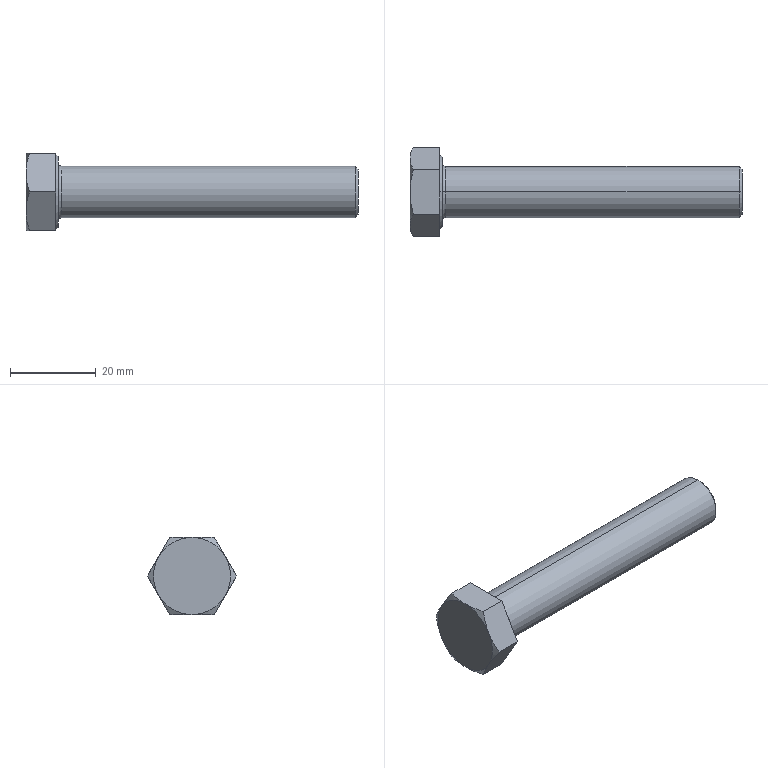Part | SolidWorks | features Chamfer 2, RevCut 2, Revolution 2, Extrusion 1, ICE 1 | 1 solid | 24 faces | box 77.5 x 20.785 x 18 mm | volume 9981 mm3 | cone 10 | plane 10 | cylinder 2 | torus 2 | commonest cylinder face diameters 12 x2
STEP:
#1=CARTESIAN_POINT('',(7.5,0.,8.215));
#2=VERTEX_POINT('',#1);
#3=CARTESIAN_POINT('',(7.5,0.,-8.215));
#4=VERTEX_POINT('',#3);
#5=CARTESIAN_POINT('',(7.5,0.,0.));
#6=DIRECTION('',(-1.,0.,0.));
#7=DIRECTION('',(0.,0.,1.));
#8=AXIS2_PLACEMENT_3D('',#5,#6,#7);
#9=CIRCLE('',#8,8.215);
#10=EDGE_CURVE('',#2,#4,#9,.T.);
#11=ORIENTED_EDGE('',*,*,#10,.T.);
#12=CARTESIAN_POINT('',(6.9,0.,-8.815));
#13=VERTEX_POINT('',#12);
#14=CARTESIAN_POINT('',(6.9,0.,-8.815));
#15=DIRECTION('',(-0.7071,0.,-0.7071));
#16=VECTOR('',#15,1000.);
#17=LINE('',#14,#16);
#18=EDGE_CURVE('',#4,#13,#17,.T.);
#19=ORIENTED_EDGE('',*,*,#18,.T.);
#20=CARTESIAN_POINT('',(6.9,0.,8.815));
#21=VERTEX_POINT('',#20);
#22=CARTESIAN_POINT('',(6.9,0.,0.));
#23=DIRECTION('',(-1.,0.,0.));
#24=DIRECTION('',(0.,0.,1.));
#25=AXIS2_PLACEMENT_3D('',#22,#23,#24);
#26=CIRCLE('',#25,8.815);
#27=EDGE_CURVE('',#21,#13,#26,.T.);
#28=ORIENTED_EDGE('',*,*,#27,.F.);
#29=CARTESIAN_POINT('',(6.9,0.,8.815));
#30=DIRECTION('',(-0.7071,0.,0.7071));
#31=VECTOR('',#30,1000.);
#32=LINE('',#29,#31);
#33=EDGE_CURVE('',#2,#21,#32,.T.);
#34=ORIENTED_EDGE('',*,*,#33,.F.);
#35=EDGE_LOOP('',(#11,#19,#28,#34));
#36=FACE_OUTER_BOUND('',#35,.T.);
#37=CARTESIAN_POINT('',(6.9,0.,0.));
#38=DIRECTION('',(-1.,0.,0.));
#39=DIRECTION('',(0.,0.,1.));
#40=AXIS2_PLACEMENT_3D('',#37,#38,#39);
#41=CONICAL_SURFACE('',#40,8.815,0.7854);
#42=ADVANCED_FACE('',(#36),#41,.T.);
#43=CARTESIAN_POINT('',(77.5,0.,-5.333));
#44=VERTEX_POINT('',#43);
#45=CARTESIAN_POINT('',(77.5,0.,5.333));
#46=VERTEX_POINT('',#45);
#47=CARTESIAN_POINT('',(77.5,0.,0.));
#48=DIRECTION('',(1.,0.,0.));
#49=DIRECTION('',(0.,0.,1.));
#50=AXIS2_PLACEMENT_3D('',#47,#48,#49);
#51=CIRCLE('',#50,5.333);
#52=EDGE_CURVE('',#44,#46,#51,.T.);
#53=ORIENTED_EDGE('',*,*,#52,.F.);
#54=CARTESIAN_POINT('',(76.833,0.,-6.));
#55=VERTEX_POINT('',#54);
#56=CARTESIAN_POINT('',(76.833,0.,-6.));
#57=DIRECTION('',(-0.7071,0.,-0.7071));
#58=VECTOR('',#57,1000.);
#59=LINE('',#56,#58);
#60=EDGE_CURVE('',#44,#55,#59,.T.);
#61=ORIENTED_EDGE('',*,*,#60,.T.);
#62=CARTESIAN_POINT('',(76.833,0.,6.));
#63=VERTEX_POINT('',#62);
#64=CARTESIAN_POINT('',(76.833,0.,0.));
#65=DIRECTION('',(-1.,0.,0.));
#66=DIRECTION('',(0.,0.,1.));
#67=AXIS2_PLACEMENT_3D('',#64,#65,#66);
#68=CIRCLE('',#67,6.);
#69=EDGE_CURVE('',#63,#55,#68,.T.);
#70=ORIENTED_EDGE('',*,*,#69,.F.);
#71=CARTESIAN_POINT('',(76.833,0.,6.));
#72=DIRECTION('',(-0.7071,0.,0.7071));
#73=VECTOR('',#72,1000.);
#74=LINE('',#71,#73);
#75=EDGE_CURVE('',#46,#63,#74,.T.);
#76=ORIENTED_EDGE('',*,*,#75,.F.);
#77=EDGE_LOOP('',(#53,#61,#70,#76));
#78=FACE_OUTER_BOUND('',#77,.T.);
#79=CARTESIAN_POINT('',(76.833,0.,0.));
#80=DIRECTION('',(-1.,0.,0.));
#81=DIRECTION('',(0.,0.,1.));
#82=AXIS2_PLACEMENT_3D('',#79,#80,#81);
#83=CONICAL_SURFACE('',#82,6.,0.7854);
#84=ADVANCED_FACE('',(#78),#83,.T.);
#85=ORIENTED_EDGE('',*,*,#69,.T.);
#86=CARTESIAN_POINT('',(8.35,0.,-6.));
#87=VERTEX_POINT('',#86);
#88=CARTESIAN_POINT('',(7.5,0.,-6.));
#89=DIRECTION('',(-1.,0.,0.));
#90=VECTOR('',#89,1000.);
#91=LINE('',#88,#90);
#92=EDGE_CURVE('',#55,#87,#91,.T.);
#93=ORIENTED_EDGE('',*,*,#92,.T.);
#94=CARTESIAN_POINT('',(8.35,0.,6.));
#95=VERTEX_POINT('',#94);
#96=CARTESIAN_POINT('',(8.35,0.,0.));
#97=DIRECTION('',(-1.,0.,0.));
#98=DIRECTION('',(0.,0.,1.));
#99=AXIS2_PLACEMENT_3D('',#96,#97,#98);
#100=CIRCLE('',#99,6.);
#101=EDGE_CURVE('',#95,#87,#100,.T.);
#102=ORIENTED_EDGE('',*,*,#101,.F.);
#103=CARTESIAN_POINT('',(7.5,0.,6.));
#104=DIRECTION('',(-1.,0.,0.));
#105=VECTOR('',#104,1000.);
#106=LINE('',#103,#105);
#107=EDGE_CURVE('',#63,#95,#106,.T.);
#108=ORIENTED_EDGE('',*,*,#107,.F.);
#109=EDGE_LOOP('',(#85,#93,#102,#108));
#110=FACE_OUTER_BOUND('',#109,.T.);
#111=CARTESIAN_POINT('',(7.5,0.,0.));
#112=DIRECTION('',(-1.,0.,0.));
#113=DIRECTION('',(0.,0.,1.));
#114=AXIS2_PLACEMENT_3D('',#111,#112,#113);
#115=CYLINDRICAL_SURFACE('',#114,6.);
#116=ADVANCED_FACE('',(#110),#115,.T.);
#117=CARTESIAN_POINT('',(7.5,0.,-6.85));
#118=VERTEX_POINT('',#117);
#119=CARTESIAN_POINT('',(7.5,0.,6.85));
#120=VERTEX_POINT('',#119);
#121=CARTESIAN_POINT('',(7.5,0.,0.));
#122=DIRECTION('',(-1.,0.,0.));
#123=DIRECTION('',(0.,0.,1.));
#124=AXIS2_PLACEMENT_3D('',#121,#122,#123);
#125=CIRCLE('',#124,6.85);
#126=EDGE_CURVE('',#118,#120,#125,.T.);
#127=ORIENTED_EDGE('',*,*,#126,.F.);
#128=CARTESIAN_POINT('',(8.35,0.,-6.85));
#129=DIRECTION('',(0.,1.,0.));
#130=DIRECTION('',(0.,0.,1.));
#131=AXIS2_PLACEMENT_3D('',#128,#129,#130);
#132=CIRCLE('',#131,0.85);
#133=EDGE_CURVE('',#118,#87,#132,.T.);
#134=ORIENTED_EDGE('',*,*,#133,.T.);
#135=CARTESIAN_POINT('',(8.35,0.,0.));
#136=DIRECTION('',(-1.,0.,0.));
#137=DIRECTION('',(0.,0.,1.));
#138=AXIS2_PLACEMENT_3D('',#135,#136,#137);
#139=CIRCLE('',#138,6.);
#140=EDGE_CURVE('',#87,#95,#139,.T.);
#141=ORIENTED_EDGE('',*,*,#140,.T.);
#142=CARTESIAN_POINT('',(8.35,0.,6.85));
#143=DIRECTION('',(0.,-1.,0.));
#144=DIRECTION('',(0.,0.,-1.));
#145=AXIS2_PLACEMENT_3D('',#142,#143,#144);
#146=CIRCLE('',#145,0.85);
#147=EDGE_CURVE('',#120,#95,#146,.T.);
#148=ORIENTED_EDGE('',*,*,#147,.F.);
#149=EDGE_LOOP('',(#127,#134,#141,#148));
#150=FACE_OUTER_BOUND('',#149,.T.);
#151=CARTESIAN_POINT('',(8.35,0.,0.));
#152=DIRECTION('',(-1.,0.,0.));
#153=DIRECTION('',(0.,0.,1.));
#154=AXIS2_PLACEMENT_3D('',#151,#152,#153);
#155=TOROIDAL_SURFACE('',#154,6.85,0.85);
#156=ADVANCED_FACE('',(#150),#155,.F.);
#157=CARTESIAN_POINT('',(7.5,0.,0.));
#158=DIRECTION('',(-1.,0.,0.));
#159=DIRECTION('',(0.,0.,1.));
#160=AXIS2_PLACEMENT_3D('',#157,#158,#159);
#161=CIRCLE('',#160,6.85);
#162=EDGE_CURVE('',#120,#118,#161,.T.);
#163=ORIENTED_EDGE('',*,*,#162,.T.);
#164=ORIENTED_EDGE('',*,*,#126,.T.);
#165=EDGE_LOOP('',(#163,#164));
#166=FACE_BOUND('',#165,.T.);
#167=ORIENTED_EDGE('',*,*,#10,.F.);
#168=CARTESIAN_POINT('',(7.5,0.,0.));
#169=DIRECTION('',(-1.,0.,0.));
#170=DIRECTION('',(0.,0.,1.));
#171=AXIS2_PLACEMENT_3D('',#168,#169,#170);
#172=CIRCLE('',#171,8.215);
#173=EDGE_CURVE('',#4,#2,#172,.T.);
#174=ORIENTED_EDGE('',*,*,#173,.F.);
#175=EDGE_LOOP('',(#167,#174));
#176=FACE_OUTER_BOUND('',#175,.T.);
#177=CARTESIAN_POINT('',(7.5,5.196,-9.));
#178=DIRECTION('',(1.,0.,0.));
#179=DIRECTION('',(0.,0.,-1.));
#180=AXIS2_PLACEMENT_3D('',#177,#178,#179);
#181=PLANE('',#180);
#182=ADVANCED_FACE('',(#166,#176),#181,.T.);
#183=ORIENTED_EDGE('',*,*,#133,.F.);
#184=ORIENTED_EDGE('',*,*,#162,.F.);
#185=ORIENTED_EDGE('',*,*,#147,.T.);
#186=ORIENTED_EDGE('',*,*,#101,.T.);
#187=EDGE_LOOP('',(#183,#184,#185,#186));
#188=FACE_OUTER_BOUND('',#187,.T.);
#189=CARTESIAN_POINT('',(8.35,0.,0.));
#190=DIRECTION('',(-1.,0.,0.));
#191=DIRECTION('',(0.,0.,1.));
#192=AXIS2_PLACEMENT_3D('',#189,#190,#191);
#193=TOROIDAL_SURFACE('',#192,6.85,0.85);
#194=ADVANCED_FACE('',(#188),#193,.F.);
#195=CARTESIAN_POINT('',(77.5,0.,0.));
#196=DIRECTION('',(1.,0.,0.));
#197=DIRECTION('',(0.,0.,1.));
#198=AXIS2_PLACEMENT_3D('',#195,#196,#197);
#199=CIRCLE('',#198,5.333);
#200=EDGE_CURVE('',#46,#44,#199,.T.);
#201=ORIENTED_EDGE('',*,*,#200,.T.);
#202=ORIENTED_EDGE('',*,*,#52,.T.);
#203=EDGE_LOOP('',(#201,#202));
#204=FACE_OUTER_BOUND('',#203,.T.);
#205=CARTESIAN_POINT('',(77.5,6.,0.));
#206=DIRECTION('',(-1.,0.,0.));
#207=DIRECTION('',(0.,0.,1.));
#208=AXIS2_PLACEMENT_3D('',#205,#206,#207);
#209=PLANE('',#208);
#210=ADVANCED_FACE('',(#204),#209,.F.);
#211=ORIENTED_EDGE('',*,*,#92,.F.);
#212=CARTESIAN_POINT('',(76.833,0.,0.));
#213=DIRECTION('',(-1.,0.,0.));
#214=DIRECTION('',(0.,0.,1.));
#215=AXIS2_PLACEMENT_3D('',#212,#213,#214);
#216=CIRCLE('',#215,6.);
#217=EDGE_CURVE('',#55,#63,#216,.T.);
#218=ORIENTED_EDGE('',*,*,#217,.T.);
#219=ORIENTED_EDGE('',*,*,#107,.T.);
#220=ORIENTED_EDGE('',*,*,#140,.F.);
#221=EDGE_LOOP('',(#211,#218,#219,#220));
#222=FACE_OUTER_BOUND('',#221,.T.);
#223=CARTESIAN_POINT('',(7.5,0.,0.));
#224=DIRECTION('',(-1.,0.,0.));
#225=DIRECTION('',(0.,0.,1.));
#226=AXIS2_PLACEMENT_3D('',#223,#224,#225);
#227=CYLINDRICAL_SURFACE('',#226,6.);
#228=ADVANCED_FACE('',(#222),#227,.T.);
#229=ORIENTED_EDGE('',*,*,#60,.F.);
#230=ORIENTED_EDGE('',*,*,#200,.F.);
#231=ORIENTED_EDGE('',*,*,#75,.T.);
#232=ORIENTED_EDGE('',*,*,#217,.F.);
#233=EDGE_LOOP('',(#229,#230,#231,#232));
#234=FACE_OUTER_BOUND('',#233,.T.);
#235=CARTESIAN_POINT('',(76.833,0.,0.));
#236=DIRECTION('',(-1.,0.,0.));
#237=DIRECTION('',(0.,0.,1.));
#238=AXIS2_PLACEMENT_3D('',#235,#236,#237);
#239=CONICAL_SURFACE('',#238,6.,0.7854);
#240=ADVANCED_FACE('',(#234),#239,.T.);
#241=ORIENTED_EDGE('',*,*,#27,.T.);
#242=CARTESIAN_POINT('',(6.9,0.,0.));
#243=DIRECTION('',(-1.,0.,0.));
#244=DIRECTION('',(0.,0.,1.));
#245=AXIS2_PLACEMENT_3D('',#242,#243,#244);
#246=CIRCLE('',#245,8.815);
#247=EDGE_CURVE('',#13,#21,#246,.T.);
#248=ORIENTED_EDGE('',*,*,#247,.T.);
#249=EDGE_LOOP('',(#241,#248));
#250=FACE_BOUND('',#249,.T.);
#251=CARTESIAN_POINT('',(6.9,-5.196,-9.));
#252=VERTEX_POINT('',#251);
#253=CARTESIAN_POINT('',(6.9,5.196,-9.));
#254=VERTEX_POINT('',#253);
#255=CARTESIAN_POINT('',(6.9,-5.196,-9.));
#256=DIRECTION('',(0.,1.,0.));
#257=VECTOR('',#256,1000.);
#258=LINE('',#255,#257);
#259=EDGE_CURVE('',#252,#254,#258,.T.);
#260=ORIENTED_EDGE('',*,*,#259,.T.);
#261=CARTESIAN_POINT('',(6.9,10.392,0.));
#262=VERTEX_POINT('',#261);
#263=CARTESIAN_POINT('',(6.9,5.196,-9.));
#264=DIRECTION('',(0.,0.5,0.866));
#265=VECTOR('',#264,1000.);
#266=LINE('',#263,#265);
#267=EDGE_CURVE('',#254,#262,#266,.T.);
#268=ORIENTED_EDGE('',*,*,#267,.T.);
#269=CARTESIAN_POINT('',(6.9,5.196,9.));
#270=VERTEX_POINT('',#269);
#271=CARTESIAN_POINT('',(6.9,10.392,0.));
#272=DIRECTION('',(0.,-0.5,0.866));
#273=VECTOR('',#272,1000.);
#274=LINE('',#271,#273);
#275=EDGE_CURVE('',#262,#270,#274,.T.);
#276=ORIENTED_EDGE('',*,*,#275,.T.);
#277=CARTESIAN_POINT('',(6.9,-5.196,9.));
#278=VERTEX_POINT('',#277);
#279=CARTESIAN_POINT('',(6.9,5.196,9.));
#280=DIRECTION('',(0.,-1.,0.));
#281=VECTOR('',#280,1000.);
#282=LINE('',#279,#281);
#283=EDGE_CURVE('',#270,#278,#282,.T.);
#284=ORIENTED_EDGE('',*,*,#283,.T.);
#285=CARTESIAN_POINT('',(6.9,-10.392,0.));
#286=VERTEX_POINT('',#285);
#287=CARTESIAN_POINT('',(6.9,-5.196,9.));
#288=DIRECTION('',(0.,-0.5,-0.866));
#289=VECTOR('',#288,1000.);
#290=LINE('',#287,#289);
#291=EDGE_CURVE('',#278,#286,#290,.T.);
#292=ORIENTED_EDGE('',*,*,#291,.T.);
#293=CARTESIAN_POINT('',(6.9,-10.392,0.));
#294=DIRECTION('',(0.,0.5,-0.866));
#295=VECTOR('',#294,1000.);
#296=LINE('',#293,#295);
#297=EDGE_CURVE('',#286,#252,#296,.T.);
#298=ORIENTED_EDGE('',*,*,#297,.T.);
#299=EDGE_LOOP('',(#260,#268,#276,#284,#292,#298));
#300=FACE_OUTER_BOUND('',#299,.T.);
#301=CARTESIAN_POINT('',(6.9,-8.815,0.));
#302=DIRECTION('',(1.,0.,0.));
#303=DIRECTION('',(0.,0.,-1.));
#304=AXIS2_PLACEMENT_3D('',#301,#302,#303);
#305=PLANE('',#304);
#306=ADVANCED_FACE('',(#250,#300),#305,.T.);
#307=ORIENTED_EDGE('',*,*,#18,.F.);
#308=ORIENTED_EDGE('',*,*,#173,.T.);
#309=ORIENTED_EDGE('',*,*,#33,.T.);
#310=ORIENTED_EDGE('',*,*,#247,.F.);
#311=EDGE_LOOP('',(#307,#308,#309,#310));
#312=FACE_OUTER_BOUND('',#311,.T.);
#313=CARTESIAN_POINT('',(6.9,0.,0.));
#314=DIRECTION('',(-1.,0.,0.));
#315=DIRECTION('',(0.,0.,1.));
#316=AXIS2_PLACEMENT_3D('',#313,#314,#315);
#317=CONICAL_SURFACE('',#316,8.815,0.7854);
#318=ADVANCED_FACE('',(#312),#317,.T.);
#319=CARTESIAN_POINT('',(0.,0.,-9.));
#320=VERTEX_POINT('',#319);
#321=CARTESIAN_POINT('',(0.,7.794,-4.5));
#322=VERTEX_POINT('',#321);
#323=CARTESIAN_POINT('',(0.,0.,0.));
#324=DIRECTION('',(1.,0.,0.));
#325=DIRECTION('',(0.,0.,-1.));
#326=AXIS2_PLACEMENT_3D('',#323,#324,#325);
#327=CIRCLE('',#326,9.);
#328=EDGE_CURVE('',#320,#322,#327,.T.);
#329=ORIENTED_EDGE('',*,*,#328,.F.);
#330=CARTESIAN_POINT('',(0.,-7.794,-4.5));
#331=VERTEX_POINT('',#330);
#332=CARTESIAN_POINT('',(0.,0.,0.));
#333=DIRECTION('',(1.,0.,0.));
#334=DIRECTION('',(0.,0.,-1.));
#335=AXIS2_PLACEMENT_3D('',#332,#333,#334);
#336=CIRCLE('',#335,9.);
#337=EDGE_CURVE('',#331,#320,#336,.T.);
#338=ORIENTED_EDGE('',*,*,#337,.F.);
#339=CARTESIAN_POINT('',(0.,-7.794,4.5));
#340=VERTEX_POINT('',#339);
#341=CARTESIAN_POINT('',(0.,0.,0.));
#342=DIRECTION('',(1.,0.,0.));
#343=DIRECTION('',(0.,0.,-1.));
#344=AXIS2_PLACEMENT_3D('',#341,#342,#343);
#345=CIRCLE('',#344,9.);
#346=EDGE_CURVE('',#340,#331,#345,.T.);
#347=ORIENTED_EDGE('',*,*,#346,.F.);
#348=CARTESIAN_POINT('',(0.,0.,9.));
#349=VERTEX_POINT('',#348);
#350=CARTESIAN_POINT('',(0.,0.,0.));
#351=DIRECTION('',(1.,0.,0.));
#352=DIRECTION('',(0.,0.,-1.));
#353=AXIS2_PLACEMENT_3D('',#350,#351,#352);
#354=CIRCLE('',#353,9.);
#355=EDGE_CURVE('',#349,#340,#354,.T.);
#356=ORIENTED_EDGE('',*,*,#355,.F.);
#357=CARTESIAN_POINT('',(0.,7.794,4.5));
#358=VERTEX_POINT('',#357);
#359=CARTESIAN_POINT('',(0.,0.,0.));
#360=DIRECTION('',(-1.,0.,0.));
#361=DIRECTION('',(0.,0.,1.));
#362=AXIS2_PLACEMENT_3D('',#359,#360,#361);
#363=CIRCLE('',#362,9.);
#364=EDGE_CURVE('',#349,#358,#363,.T.);
#365=ORIENTED_EDGE('',*,*,#364,.T.);
#366=CARTESIAN_POINT('',(0.,0.,0.));
#367=DIRECTION('',(1.,0.,0.));
#368=DIRECTION('',(0.,0.,-1.));
#369=AXIS2_PLACEMENT_3D('',#366,#367,#368);
#370=CIRCLE('',#369,9.);
#371=EDGE_CURVE('',#322,#358,#370,.T.);
#372=ORIENTED_EDGE('',*,*,#371,.F.);
#373=EDGE_LOOP('',(#329,#338,#347,#356,#365,#372));
#374=FACE_OUTER_BOUND('',#373,.T.);
#375=CARTESIAN_POINT('',(0.,5.196,-9.));
#376=DIRECTION('',(1.,0.,0.));
#377=DIRECTION('',(0.,0.,-1.));
#378=AXIS2_PLACEMENT_3D('',#375,#376,#377);
#379=PLANE('',#378);
#380=ADVANCED_FACE('',(#374),#379,.F.);
#381=CARTESIAN_POINT('',(0.8038,5.196,-9.));
#382=VERTEX_POINT('',#381);
#383=CARTESIAN_POINT('',(0.,7.794,-4.5));
#384=CARTESIAN_POINT('',(0.,7.574,-4.882));
#385=CARTESIAN_POINT('',(0.019,7.352,-5.266));
#386=CARTESIAN_POINT('',(0.09253,6.914,-6.024));
#387=CARTESIAN_POINT('',(0.147,6.697,-6.401));
#388=CARTESIAN_POINT('',(0.357,6.048,-7.525));
#389=CARTESIAN_POINT('',(0.5591,5.62,-8.266));
#390=CARTESIAN_POINT('',(0.8038,5.196,-9.));
#391=B_SPLINE_CURVE_WITH_KNOTS('',3,(#383,#384,#385,#386,#387,#388,#389,#390),.UNSPECIFIED.,.F.,.F.,(4,2,2,4),(0.005258,0.006567,0.007877,0.0105),.UNSPECIFIED.);
#392=EDGE_CURVE('',#322,#382,#391,.T.);
#393=ORIENTED_EDGE('',*,*,#392,.T.);
#394=CARTESIAN_POINT('',(0.8038,5.196,-9.));
#395=CARTESIAN_POINT('',(0.5613,4.356,-9.));
#396=CARTESIAN_POINT('',(0.3593,3.505,-9.));
#397=CARTESIAN_POINT('',(0.07758,1.769,-9.));
#398=CARTESIAN_POINT('',(0.,0.8787,-9.));
#399=CARTESIAN_POINT('',(0.,0.,-9.));
#400=B_SPLINE_CURVE_WITH_KNOTS('',3,(#394,#395,#396,#397,#398,#399),.UNSPECIFIED.,.F.,.F.,(4,2,4),(0.003787,0.00641,0.009033),.UNSPECIFIED.);
#401=EDGE_CURVE('',#382,#320,#400,.T.);
#402=ORIENTED_EDGE('',*,*,#401,.T.);
#403=ORIENTED_EDGE('',*,*,#328,.T.);
#404=EDGE_LOOP('',(#393,#402,#403));
#405=FACE_OUTER_BOUND('',#404,.T.);
#406=CARTESIAN_POINT('',(0.,0.,0.));
#407=DIRECTION('',(1.,0.,0.));
#408=DIRECTION('',(0.,0.,1.));
#409=AXIS2_PLACEMENT_3D('',#406,#407,#408);
#410=CONICAL_SURFACE('',#409,9.,1.047);
#411=ADVANCED_FACE('',(#405),#410,.T.);
#412=CARTESIAN_POINT('',(0.8038,10.392,0.));
#413=VERTEX_POINT('',#412);
#414=CARTESIAN_POINT('',(0.,7.794,4.5));
#415=CARTESIAN_POINT('',(0.,8.015,4.118));
#416=CARTESIAN_POINT('',(0.019,8.236,3.734));
#417=CARTESIAN_POINT('',(0.09253,8.674,2.976));
#418=CARTESIAN_POINT('',(0.147,8.892,2.599));
#419=CARTESIAN_POINT('',(0.357,9.541,1.475));
#420=CARTESIAN_POINT('',(0.5591,9.968,0.7343));
#421=CARTESIAN_POINT('',(0.8038,10.392,0.));
#422=B_SPLINE_CURVE_WITH_KNOTS('',3,(#414,#415,#416,#417,#418,#419,#420,#421),.UNSPECIFIED.,.F.,.F.,(4,2,2,4),(0.005258,0.006567,0.007877,0.0105),.UNSPECIFIED.);
#423=EDGE_CURVE('',#358,#413,#422,.T.);
#424=ORIENTED_EDGE('',*,*,#423,.T.);
#425=CARTESIAN_POINT('',(0.8038,10.392,0.));
#426=CARTESIAN_POINT('',(0.5585,9.967,-0.7361));
#427=CARTESIAN_POINT('',(0.3563,9.539,-1.478));
#428=CARTESIAN_POINT('',(0.07661,8.674,-2.976));
#429=CARTESIAN_POINT('',(0.,8.237,-3.733));
#430=CARTESIAN_POINT('',(0.,7.794,-4.5));
#431=B_SPLINE_CURVE_WITH_KNOTS('',3,(#425,#426,#427,#428,#429,#430),.UNSPECIFIED.,.F.,.F.,(4,2,4),(0.000000238,0.002629,0.005258),.UNSPECIFIED.);
#432=EDGE_CURVE('',#413,#322,#431,.T.);
#433=ORIENTED_EDGE('',*,*,#432,.T.);
#434=ORIENTED_EDGE('',*,*,#371,.T.);
#435=EDGE_LOOP('',(#424,#433,#434));
#436=FACE_OUTER_BOUND('',#435,.T.);
#437=CARTESIAN_POINT('',(0.,0.,0.));
#438=DIRECTION('',(1.,0.,0.));
#439=DIRECTION('',(0.,0.,1.));
#440=AXIS2_PLACEMENT_3D('',#437,#438,#439);
#441=CONICAL_SURFACE('',#440,9.,1.047);
#442=ADVANCED_FACE('',(#436),#441,.T.);
#443=CARTESIAN_POINT('',(0.8038,5.196,9.));
#444=VERTEX_POINT('',#443);
#445=CARTESIAN_POINT('',(0.8038,5.196,9.));
#446=CARTESIAN_POINT('',(0.5585,5.621,8.264));
#447=CARTESIAN_POINT('',(0.3563,6.049,7.522));
#448=CARTESIAN_POINT('',(0.07661,6.914,6.024));
#449=CARTESIAN_POINT('',(0.,7.352,5.267));
#450=CARTESIAN_POINT('',(0.,7.794,4.5));
#451=B_SPLINE_CURVE_WITH_KNOTS('',3,(#445,#446,#447,#448,#449,#450),.UNSPECIFIED.,.F.,.F.,(4,2,4),(0.000000238,0.002629,0.005258),.UNSPECIFIED.);
#452=EDGE_CURVE('',#444,#358,#451,.T.);
#453=ORIENTED_EDGE('',*,*,#452,.T.);
#454=ORIENTED_EDGE('',*,*,#364,.F.);
#455=CARTESIAN_POINT('',(0.,0.,9.));
#456=CARTESIAN_POINT('',(0.,0.8787,9.));
#457=CARTESIAN_POINT('',(0.07758,1.769,9.));
#458=CARTESIAN_POINT('',(0.3593,3.505,9.));
#459=CARTESIAN_POINT('',(0.5613,4.356,9.));
#460=CARTESIAN_POINT('',(0.8038,5.196,9.));
#461=B_SPLINE_CURVE_WITH_KNOTS('',3,(#455,#456,#457,#458,#459,#460),.UNSPECIFIED.,.F.,.F.,(4,2,4),(0.01455,0.01718,0.01981),.UNSPECIFIED.);
#462=EDGE_CURVE('',#349,#444,#461,.T.);
#463=ORIENTED_EDGE('',*,*,#462,.T.);
#464=EDGE_LOOP('',(#453,#454,#463));
#465=FACE_OUTER_BOUND('',#464,.T.);
#466=CARTESIAN_POINT('',(0.,0.,0.));
#467=DIRECTION('',(1.,0.,0.));
#468=DIRECTION('',(0.,0.,1.));
#469=AXIS2_PLACEMENT_3D('',#466,#467,#468);
#470=CONICAL_SURFACE('',#469,9.,1.047);
#471=ADVANCED_FACE('',(#465),#470,.T.);
#472=CARTESIAN_POINT('',(0.8038,-5.196,9.));
#473=VERTEX_POINT('',#472);
#474=CARTESIAN_POINT('',(0.8038,-5.196,9.));
#475=CARTESIAN_POINT('',(0.5599,-4.351,9.));
#476=CARTESIAN_POINT('',(0.3553,-3.485,9.));
#477=CARTESIAN_POINT('',(0.07548,-1.75,9.));
#478=CARTESIAN_POINT('',(0.,-0.8781,9.));
#479=CARTESIAN_POINT('',(0.,0.,9.));
#480=B_SPLINE_CURVE_WITH_KNOTS('',3,(#474,#475,#476,#477,#478,#479),.UNSPECIFIED.,.F.,.F.,(4,2,4),(0.009291,0.01192,0.01455),.UNSPECIFIED.);
#481=EDGE_CURVE('',#473,#349,#480,.T.);
#482=ORIENTED_EDGE('',*,*,#481,.T.);
#483=ORIENTED_EDGE('',*,*,#355,.T.);
#484=CARTESIAN_POINT('',(0.,-7.794,4.5));
#485=CARTESIAN_POINT('',(0.,-7.574,4.882));
#486=CARTESIAN_POINT('',(0.019,-7.352,5.266));
#487=CARTESIAN_POINT('',(0.09253,-6.914,6.024));
#488=CARTESIAN_POINT('',(0.147,-6.697,6.401));
#489=CARTESIAN_POINT('',(0.357,-6.048,7.525));
#490=CARTESIAN_POINT('',(0.5591,-5.62,8.266));
#491=CARTESIAN_POINT('',(0.8038,-5.196,9.));
#492=B_SPLINE_CURVE_WITH_KNOTS('',3,(#484,#485,#486,#487,#488,#489,#490,#491),.UNSPECIFIED.,.F.,.F.,(4,2,2,4),(0.005258,0.006567,0.007877,0.0105),.UNSPECIFIED.);
#493=EDGE_CURVE('',#340,#473,#492,.T.);
#494=ORIENTED_EDGE('',*,*,#493,.T.);
#495=EDGE_LOOP('',(#482,#483,#494));
#496=FACE_OUTER_BOUND('',#495,.T.);
#497=CARTESIAN_POINT('',(0.,0.,0.));
#498=DIRECTION('',(1.,0.,0.));
#499=DIRECTION('',(0.,0.,1.));
#500=AXIS2_PLACEMENT_3D('',#497,#498,#499);
#501=CONICAL_SURFACE('',#500,9.,1.047);
#502=ADVANCED_FACE('',(#496),#501,.T.);
#503=CARTESIAN_POINT('',(0.8038,-5.196,-9.));
#504=VERTEX_POINT('',#503);
#505=CARTESIAN_POINT('',(0.,0.,-9.));
#506=CARTESIAN_POINT('',(0.,-0.8781,-9.));
#507=CARTESIAN_POINT('',(0.07548,-1.75,-9.));
#508=CARTESIAN_POINT('',(0.3553,-3.485,-9.));
#509=CARTESIAN_POINT('',(0.5599,-4.351,-9.));
#510=CARTESIAN_POINT('',(0.8038,-5.196,-9.));
#511=B_SPLINE_CURVE_WITH_KNOTS('',3,(#505,#506,#507,#508,#509,#510),.UNSPECIFIED.,.F.,.F.,(4,2,4),(0.009033,0.01165,0.01428),.UNSPECIFIED.);
#512=EDGE_CURVE('',#320,#504,#511,.T.);
#513=ORIENTED_EDGE('',*,*,#512,.T.);
#514=CARTESIAN_POINT('',(0.8038,-5.196,-9.));
#515=CARTESIAN_POINT('',(0.5585,-5.621,-8.264));
#516=CARTESIAN_POINT('',(0.3563,-6.049,-7.522));
#517=CARTESIAN_POINT('',(0.07661,-6.914,-6.024));
#518=CARTESIAN_POINT('',(0.,-7.352,-5.267));
#519=CARTESIAN_POINT('',(0.,-7.794,-4.5));
#520=B_SPLINE_CURVE_WITH_KNOTS('',3,(#514,#515,#516,#517,#518,#519),.UNSPECIFIED.,.F.,.F.,(4,2,4),(0.000000238,0.002629,0.005258),.UNSPECIFIED.);
#521=EDGE_CURVE('',#504,#331,#520,.T.);
#522=ORIENTED_EDGE('',*,*,#521,.T.);
#523=ORIENTED_EDGE('',*,*,#337,.T.);
#524=EDGE_LOOP('',(#513,#522,#523));
#525=FACE_OUTER_BOUND('',#524,.T.);
#526=CARTESIAN_POINT('',(0.,0.,0.));
#527=DIRECTION('',(1.,0.,0.));
#528=DIRECTION('',(0.,0.,1.));
#529=AXIS2_PLACEMENT_3D('',#526,#527,#528);
#530=CONICAL_SURFACE('',#529,9.,1.047);
#531=ADVANCED_FACE('',(#525),#530,.T.);
#532=CARTESIAN_POINT('',(0.8038,-10.392,0.));
#533=VERTEX_POINT('',#532);
#534=CARTESIAN_POINT('',(0.8038,-10.392,0.));
#535=CARTESIAN_POINT('',(0.5585,-9.967,0.7361));
#536=CARTESIAN_POINT('',(0.3563,-9.539,1.478));
#537=CARTESIAN_POINT('',(0.07661,-8.674,2.976));
#538=CARTESIAN_POINT('',(0.,-8.237,3.733));
#539=CARTESIAN_POINT('',(0.,-7.794,4.5));
#540=B_SPLINE_CURVE_WITH_KNOTS('',3,(#534,#535,#536,#537,#538,#539),.UNSPECIFIED.,.F.,.F.,(4,2,4),(0.000000238,0.002629,0.005258),.UNSPECIFIED.);
#541=EDGE_CURVE('',#533,#340,#540,.T.);
#542=ORIENTED_EDGE('',*,*,#541,.T.);
#543=ORIENTED_EDGE('',*,*,#346,.T.);
#544=CARTESIAN_POINT('',(0.,-7.794,-4.5));
#545=CARTESIAN_POINT('',(0.,-8.015,-4.118));
#546=CARTESIAN_POINT('',(0.019,-8.236,-3.734));
#547=CARTESIAN_POINT('',(0.09253,-8.674,-2.976));
#548=CARTESIAN_POINT('',(0.147,-8.892,-2.599));
#549=CARTESIAN_POINT('',(0.357,-9.541,-1.475));
#550=CARTESIAN_POINT('',(0.5591,-9.968,-0.7343));
#551=CARTESIAN_POINT('',(0.8038,-10.392,0.));
#552=B_SPLINE_CURVE_WITH_KNOTS('',3,(#544,#545,#546,#547,#548,#549,#550,#551),.UNSPECIFIED.,.F.,.F.,(4,2,2,4),(0.005258,0.006567,0.007877,0.0105),.UNSPECIFIED.);
#553=EDGE_CURVE('',#331,#533,#552,.T.);
#554=ORIENTED_EDGE('',*,*,#553,.T.);
#555=EDGE_LOOP('',(#542,#543,#554));
#556=FACE_OUTER_BOUND('',#555,.T.);
#557=CARTESIAN_POINT('',(0.,0.,0.));
#558=DIRECTION('',(1.,0.,0.));
#559=DIRECTION('',(0.,0.,1.));
#560=AXIS2_PLACEMENT_3D('',#557,#558,#559);
#561=CONICAL_SURFACE('',#560,9.,1.047);
#562=ADVANCED_FACE('',(#556),#561,.T.);
#563=ORIENTED_EDGE('',*,*,#297,.F.);
#564=CARTESIAN_POINT('',(7.5,-10.392,0.));
#565=DIRECTION('',(-1.,0.,0.));
#566=VECTOR('',#565,1000.);
#567=LINE('',#564,#566);
#568=EDGE_CURVE('',#286,#533,#567,.T.);
#569=ORIENTED_EDGE('',*,*,#568,.T.);
#570=ORIENTED_EDGE('',*,*,#553,.F.);
#571=ORIENTED_EDGE('',*,*,#521,.F.);
#572=CARTESIAN_POINT('',(7.5,-5.196,-9.));
#573=DIRECTION('',(-1.,0.,0.));
#574=VECTOR('',#573,1000.);
#575=LINE('',#572,#574);
#576=EDGE_CURVE('',#252,#504,#575,.T.);
#577=ORIENTED_EDGE('',*,*,#576,.F.);
#578=EDGE_LOOP('',(#563,#569,#570,#571,#577));
#579=FACE_OUTER_BOUND('',#578,.T.);
#580=CARTESIAN_POINT('',(7.5,-10.392,0.));
#581=DIRECTION('',(0.,0.866,0.5));
#582=DIRECTION('',(0.,-0.5,0.866));
#583=AXIS2_PLACEMENT_3D('',#580,#581,#582);
#584=PLANE('',#583);
#585=ADVANCED_FACE('',(#579),#584,.F.);
#586=ORIENTED_EDGE('',*,*,#291,.F.);
#587=CARTESIAN_POINT('',(7.5,-5.196,9.));
#588=DIRECTION('',(-1.,0.,0.));
#589=VECTOR('',#588,1000.);
#590=LINE('',#587,#589);
#591=EDGE_CURVE('',#278,#473,#590,.T.);
#592=ORIENTED_EDGE('',*,*,#591,.T.);
#593=ORIENTED_EDGE('',*,*,#493,.F.);
#594=ORIENTED_EDGE('',*,*,#541,.F.);
#595=ORIENTED_EDGE('',*,*,#568,.F.);
#596=EDGE_LOOP('',(#586,#592,#593,#594,#595));
#597=FACE_OUTER_BOUND('',#596,.T.);
#598=CARTESIAN_POINT('',(7.5,-5.196,9.));
#599=DIRECTION('',(0.,0.866,-0.5));
#600=DIRECTION('',(0.,0.5,0.866));
#601=AXIS2_PLACEMENT_3D('',#598,#599,#600);
#602=PLANE('',#601);
#603=ADVANCED_FACE('',(#597),#602,.F.);
#604=ORIENTED_EDGE('',*,*,#283,.F.);
#605=CARTESIAN_POINT('',(7.5,5.196,9.));
#606=DIRECTION('',(-1.,0.,0.));
#607=VECTOR('',#606,1000.);
#608=LINE('',#605,#607);
#609=EDGE_CURVE('',#270,#444,#608,.T.);
#610=ORIENTED_EDGE('',*,*,#609,.T.);
#611=ORIENTED_EDGE('',*,*,#462,.F.);
#612=ORIENTED_EDGE('',*,*,#481,.F.);
#613=ORIENTED_EDGE('',*,*,#591,.F.);
#614=EDGE_LOOP('',(#604,#610,#611,#612,#613));
#615=FACE_OUTER_BOUND('',#614,.T.);
#616=CARTESIAN_POINT('',(7.5,5.196,9.));
#617=DIRECTION('',(0.,0.,-1.));
#618=DIRECTION('',(0.,1.,0.));
#619=AXIS2_PLACEMENT_3D('',#616,#617,#618);
#620=PLANE('',#619);
#621=ADVANCED_FACE('',(#615),#620,.F.);
#622=ORIENTED_EDGE('',*,*,#275,.F.);
#623=CARTESIAN_POINT('',(7.5,10.392,0.));
#624=DIRECTION('',(-1.,0.,0.));
#625=VECTOR('',#624,1000.);
#626=LINE('',#623,#625);
#627=EDGE_CURVE('',#262,#413,#626,.T.);
#628=ORIENTED_EDGE('',*,*,#627,.T.);
#629=ORIENTED_EDGE('',*,*,#423,.F.);
#630=ORIENTED_EDGE('',*,*,#452,.F.);
#631=ORIENTED_EDGE('',*,*,#609,.F.);
#632=EDGE_LOOP('',(#622,#628,#629,#630,#631));
#633=FACE_OUTER_BOUND('',#632,.T.);
#634=CARTESIAN_POINT('',(7.5,10.392,0.));
#635=DIRECTION('',(0.,-0.866,-0.5));
#636=DIRECTION('',(0.,0.5,-0.866));
#637=AXIS2_PLACEMENT_3D('',#634,#635,#636);
#638=PLANE('',#637);
#639=ADVANCED_FACE('',(#633),#638,.F.);
#640=ORIENTED_EDGE('',*,*,#267,.F.);
#641=CARTESIAN_POINT('',(7.5,5.196,-9.));
#642=DIRECTION('',(-1.,0.,0.));
#643=VECTOR('',#642,1000.);
#644=LINE('',#641,#643);
#645=EDGE_CURVE('',#254,#382,#644,.T.);
#646=ORIENTED_EDGE('',*,*,#645,.T.);
#647=ORIENTED_EDGE('',*,*,#392,.F.);
#648=ORIENTED_EDGE('',*,*,#432,.F.);
#649=ORIENTED_EDGE('',*,*,#627,.F.);
#650=EDGE_LOOP('',(#640,#646,#647,#648,#649));
#651=FACE_OUTER_BOUND('',#650,.T.);
#652=CARTESIAN_POINT('',(7.5,5.196,-9.));
#653=DIRECTION('',(0.,-0.866,0.5));
#654=DIRECTION('',(0.,-0.5,-0.866));
#655=AXIS2_PLACEMENT_3D('',#652,#653,#654);
#656=PLANE('',#655);
#657=ADVANCED_FACE('',(#651),#656,.F.);
#658=ORIENTED_EDGE('',*,*,#259,.F.);
#659=ORIENTED_EDGE('',*,*,#576,.T.);
#660=ORIENTED_EDGE('',*,*,#512,.F.);
#661=ORIENTED_EDGE('',*,*,#401,.F.);
#662=ORIENTED_EDGE('',*,*,#645,.F.);
#663=EDGE_LOOP('',(#658,#659,#660,#661,#662));
#664=FACE_OUTER_BOUND('',#663,.T.);
#665=CARTESIAN_POINT('',(7.5,-5.196,-9.));
#666=DIRECTION('',(0.,0.,1.));
#667=DIRECTION('',(0.,-1.,0.));
#668=AXIS2_PLACEMENT_3D('',#665,#666,#667);
#669=PLANE('',#668);
#670=ADVANCED_FACE('',(#664),#669,.F.);
#671=CLOSED_SHELL('',(#42,#84,#116,#156,#182,#194,#210,#228,#240,#306,#318,#380,#411,#442,#471,#502,#531,#562,#585,#603,#621,#639,#657,#670));
#672=MANIFOLD_SOLID_BREP('',#671);
#673=CARTESIAN_POINT('',(0.,0.,0.));
#674=DIRECTION('',(0.,0.,1.));
#675=DIRECTION('',(1.,0.,0.));
#676=AXIS2_PLACEMENT_3D('',#673,#674,#675);
#677=(LENGTH_UNIT()NAMED_UNIT(*)SI_UNIT(.MILLI.,.METRE.));
#678=UNCERTAINTY_MEASURE_WITH_UNIT(LENGTH_MEASURE(0.00001),#677,'','');
#679=(NAMED_UNIT(*)PLANE_ANGLE_UNIT()SI_UNIT($,.RADIAN.));
#680=(NAMED_UNIT(*)SI_UNIT($,.STERADIAN.)SOLID_ANGLE_UNIT());
#681=(GEOMETRIC_REPRESENTATION_CONTEXT(3)GLOBAL_UNCERTAINTY_ASSIGNED_CONTEXT((#678))GLOBAL_UNIT_ASSIGNED_CONTEXT((#677,#679,#680))REPRESENTATION_CONTEXT('',''));
#682=ADVANCED_BREP_SHAPE_REPRESENTATION('',(#672,#676),#681);